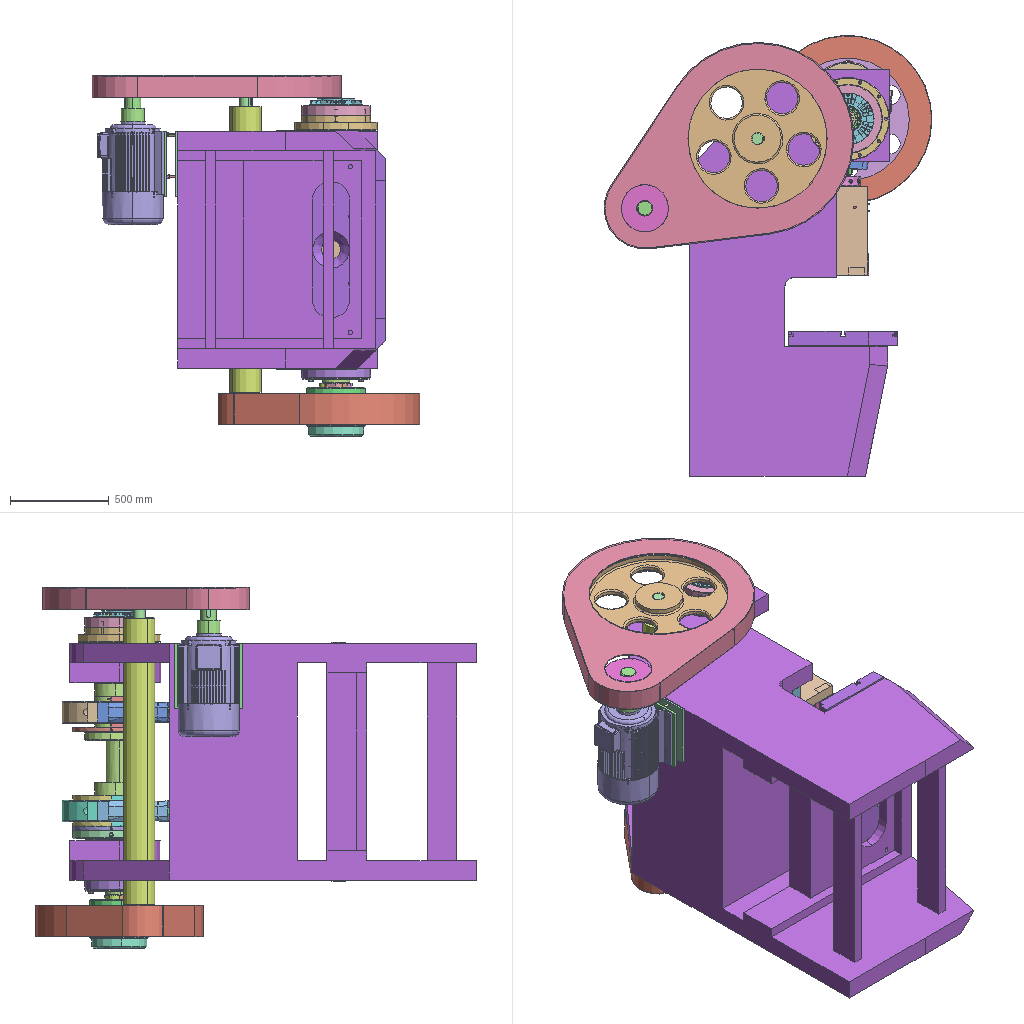Assembly | SolidWorks | 108 different items | 124 placed | box 1659 x 2230 x 1826 mm
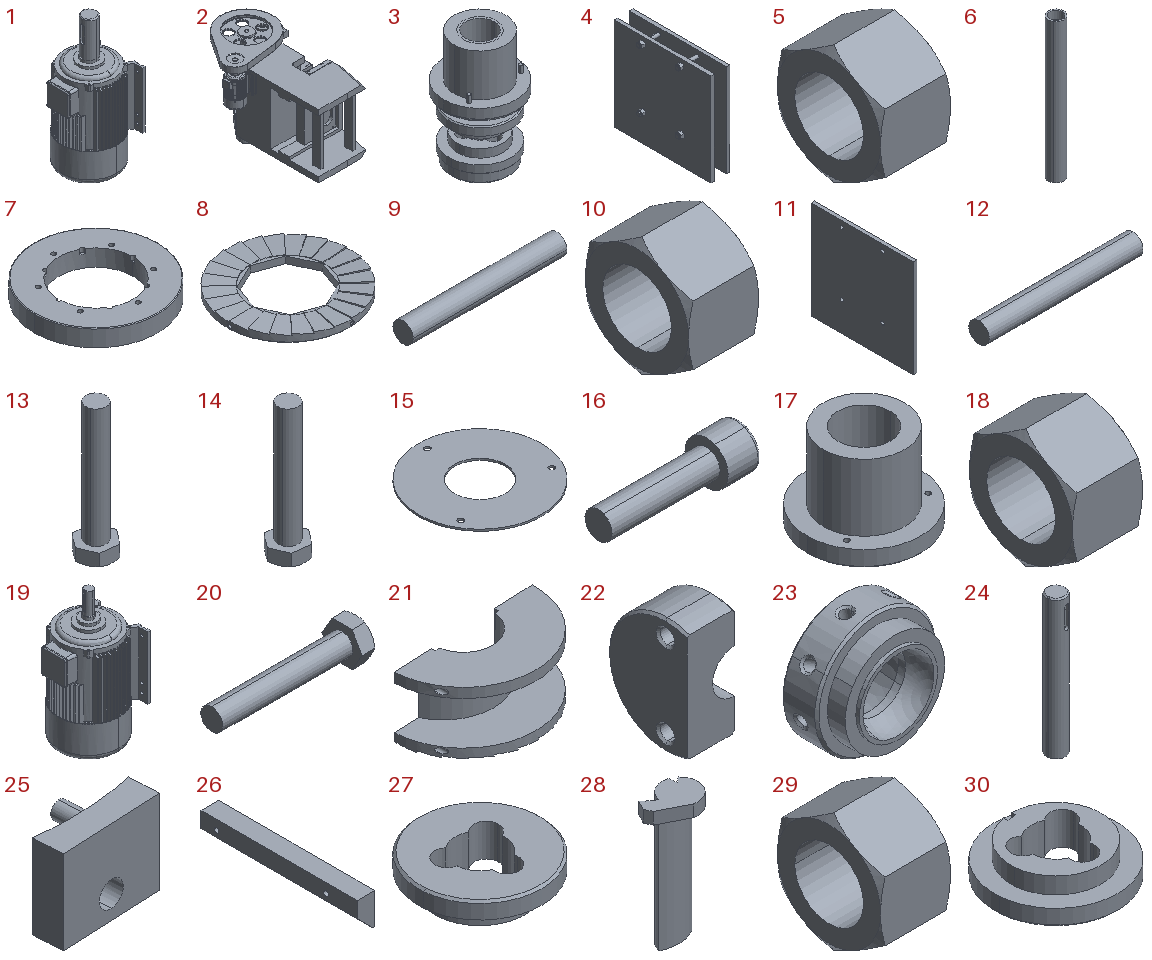Parts list (item | name | quantity | parent item | size | volume | features):
1 | (subassembly) | x1 | in 2 | 340 x 314 x 732 mm | 11771559 mm3 | -
2 | (subassembly) | x1 | - | - | 951819714 mm3 | -
3 | (subassembly) | x1 | in 2 | 350 x 350 x 550 mm | 23094575 mm3 | -
4 | (subassembly) | x1 | in 2 | 90.963 x 344.147 x 330 mm | 2772183 mm3 | -
5 | - | x1 | in 4 | 12.2 x 18 x 20.785 mm | 2031 mm3 | features BaseBody 1
6 | - | x1 | in 2 | 160 x 160 x 1444 mm | 21949365 mm3 | features BaseBody 1
7 | - | x1 | - | 350 x 350 x 48 mm | 2905895 mm3 | features HoleWzd 3, Revolution 1
8 | - | x1 | in 2 | 370 x 370 x 24.255 mm | 1594243 mm3 | features BaseBody 1
9 | - | x1 | in 4 | 90.963 x 12 x 12 mm | 10288 mm3 | features BaseBody 1
10 | - | x1 | in 4 | 12.2 x 18 x 20.785 mm | 2031 mm3 | features BaseBody 1
11 | - | x1 | in 4 | 12 x 344.147 x 330 mm | 1357393 mm3 | features BaseBody 1
12 | - | x1 | in 4 | 90.963 x 12 x 12 mm | 10288 mm3 | features BaseBody 1
13 | - | x1 | in 3 | 27.477 x 25.599 x 100 mm | 20878 mm3 | features BaseBody 1
14 | - | x1 | in 3 | 27.477 x 25.599 x 100 mm | 20878 mm3 | features BaseBody 1
15 | - | x1 | in 3 | 340 x 340 x 5 mm | 374340 mm3 | features BaseBody 1
16 | - | x1 | in 2 | 26 x 8 x 8 mm | 606.379 mm3 | features BaseBody 1
17 | - | x1 | in 3 | 350 x 350 x 255 mm | 9479362 mm3 | features BaseBody 1
18 | - | x1 | in 4 | 12.2 x 18 x 20.785 mm | 2031 mm3 | features BaseBody 1
19 | - | x1 | in 1 | 340 x 314 x 660 mm | 8782416 mm3 | features BaseBody 1
20 | - | x1 | in 2 | 100 x 27.713 x 24 mm | 20878 mm3 | features BaseBody 1
21 | - | x1 | in 2 | 369.799 x 193.623 x 159.255 mm | 2559230 mm3 | features BaseBody 1
22 | - | x1 | in 2 | 65 x 110 x 160 mm | 821212 mm3 | features BaseBody 1
23 | - | x1 | in 2 | 170 x 80 x 170 mm | 1005537 mm3 | features BaseBody 1
24 | - | x1 | in 1 | 80 x 80 x 600 mm | 2989143 mm3 | features BaseBody 1
25 | - | x1 | in 2 | 60.748 x 31.599 x 50 mm | 45964 mm3 | features BaseBody 1
26 | - | x1 | in 2 | 60 x 500 x 100 mm | 2348382 mm3 | features BaseBody 1
27 | - | x1 | in 3 | 300 x 300 x 80 mm | 3048135 mm3 | features BaseBody 1
28 | - | x1 | in 3 | 86.498 x 60 x 220 mm | 320268 mm3 | features BaseBody 1
29 | - | x1 | in 4 | 12.2 x 18 x 20.785 mm | 2031 mm3 | features BaseBody 1
30 | - | x1 | in 3 | 300 x 300 x 80 mm | 3048135 mm3 | features BaseBody 1
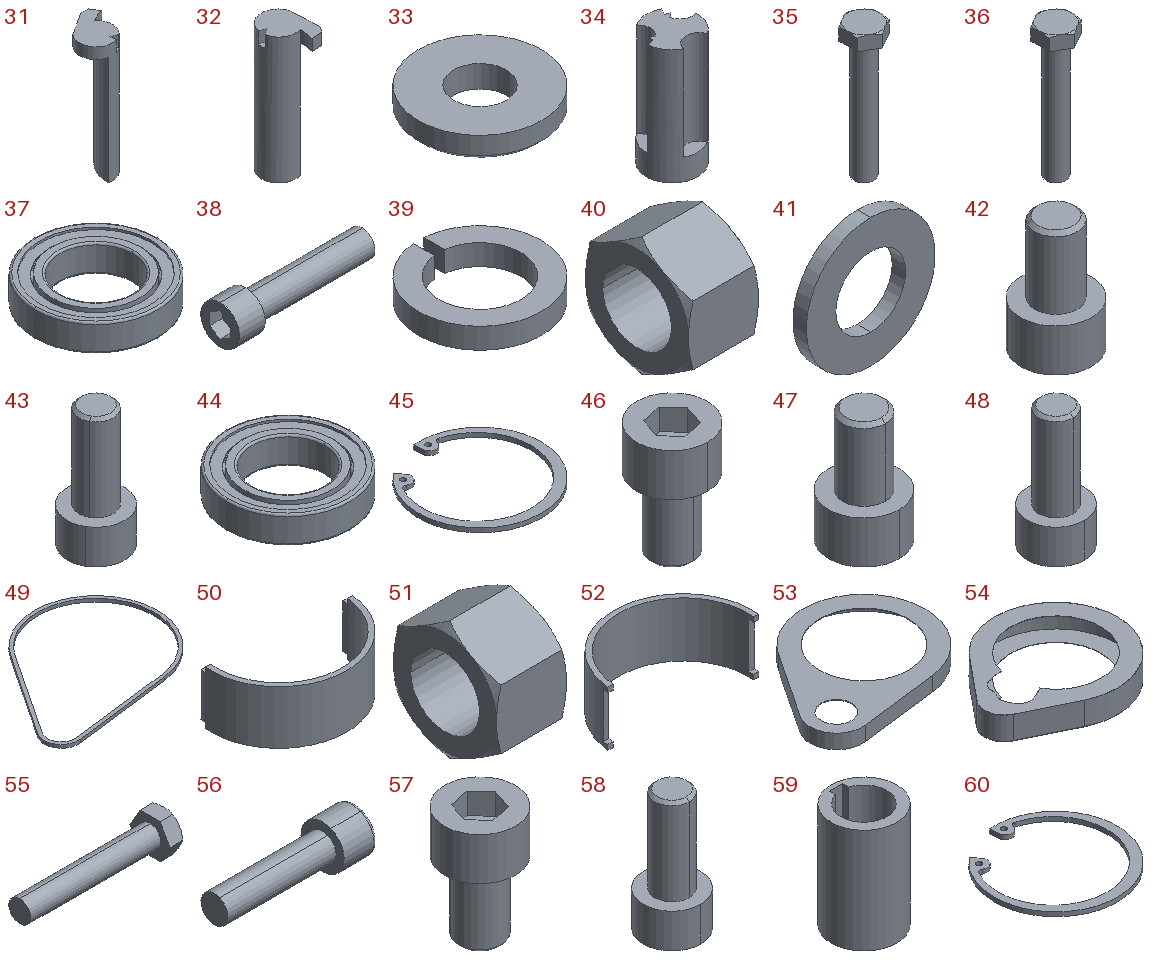31 | - | x1 | in 3 | 72.203 x 77.473 x 220 mm | 320268 mm3 | features BaseBody 1
32 | - | x1 | in 3 | 61.158 x 82.258 x 220 mm | 320268 mm3 | features BaseBody 1
33 | - | x1 | in 3 | 280 x 280 x 50 mm | 2470339 mm3 | features BaseBody 1
34 | - | x1 | in 3 | 120 x 120 x 270 mm | 2222971 mm3 | features BaseBody 1
35 | - | x1 | in 2 | 24 x 27.713 x 100 mm | 20878 mm3 | features BaseBody 1
36 | - | x1 | in 2 | 24 x 27.713 x 100 mm | 20878 mm3 | features BaseBody 1
37 | - | x1 | in 2 | 136 x 136 x 30 mm | 181462 mm3 | features BaseBody 1
38 | - | x2 | in 2 | 67 x 18 x 18 mm | 8742 mm3 | features BaseBody 1
39 | - | x2 | in 2 | 18.367 x 18.334 x 3.1 mm | 444.091 mm3 | features BaseBody 1
40 | - | x1 | in 4 | 12.2 x 18 x 20.785 mm | 2031 mm3 | features BaseBody 1
41 | - | x2 | in 2 | 24 x 2.5 x 24 mm | 799.143 mm3 | features BaseBody 1
42 | - | x7 | in 2 | 20 x 20 x 32 mm | 5504 mm3 | features BaseBody 1
43 | - | x2 | in 2 | 20 x 20 x 42 mm | 6635 mm3 | features BaseBody 1
44 | - | x1 | in 2 | 136 x 136 x 30 mm | 182204 mm3 | features BaseBody 1
45 | - | x1 | in 2 | 145 x 145 x 5 mm | 18463 mm3 | features BaseBody 1
46 | - | x1 | in 2 | 20 x 20 x 32 mm | 5504 mm3 | features BaseBody 1
47 | - | x1 | in 2 | 20 x 20 x 32 mm | 5504 mm3 | features BaseBody 1
48 | - | x1 | in 2 | 20 x 20 x 42 mm | 6635 mm3 | features BaseBody 1
49 | - | x1 | in 2 | 1063 x 845.491 x 20 mm | 1178269 mm3 | features BaseBody 1
50 | - | x1 | in 2 | 279.978 x 162.405 x 110 mm | 484543 mm3 | features BaseBody 1
51 | - | x1 | in 4 | 12.2 x 18 x 20.785 mm | 2031 mm3 | features BaseBody 1
52 | - | x1 | in 2 | 279.443 x 152.477 x 110 mm | 448510 mm3 | features BaseBody 1
53 | - | x1 | in 2 | 1263 x 1045 x 113 mm | 4506392 mm3 | features BaseBody 1
54 | - | x1 | in 2 | 1017 x 850 x 160 mm | 2046242 mm3 | features BaseBody 1
55 | - | x1 | in 2 | 100 x 27.713 x 24 mm | 20878 mm3 | features BaseBody 1
56 | - | x1 | in 2 | 26 x 8 x 8 mm | 606.379 mm3 | features BaseBody 1
57 | - | x1 | in 2 | 20 x 20 x 32 mm | 5504 mm3 | features BaseBody 1
58 | - | x1 | in 2 | 20 x 20 x 42 mm | 6635 mm3 | features BaseBody 1
59 | - | x1 | in 2 | 80 x 80 x 128 mm | 313826 mm3 | features BaseBody 1
60 | - | x1 | in 2 | 145 x 145 x 5 mm | 18463 mm3 | features BaseBody 1
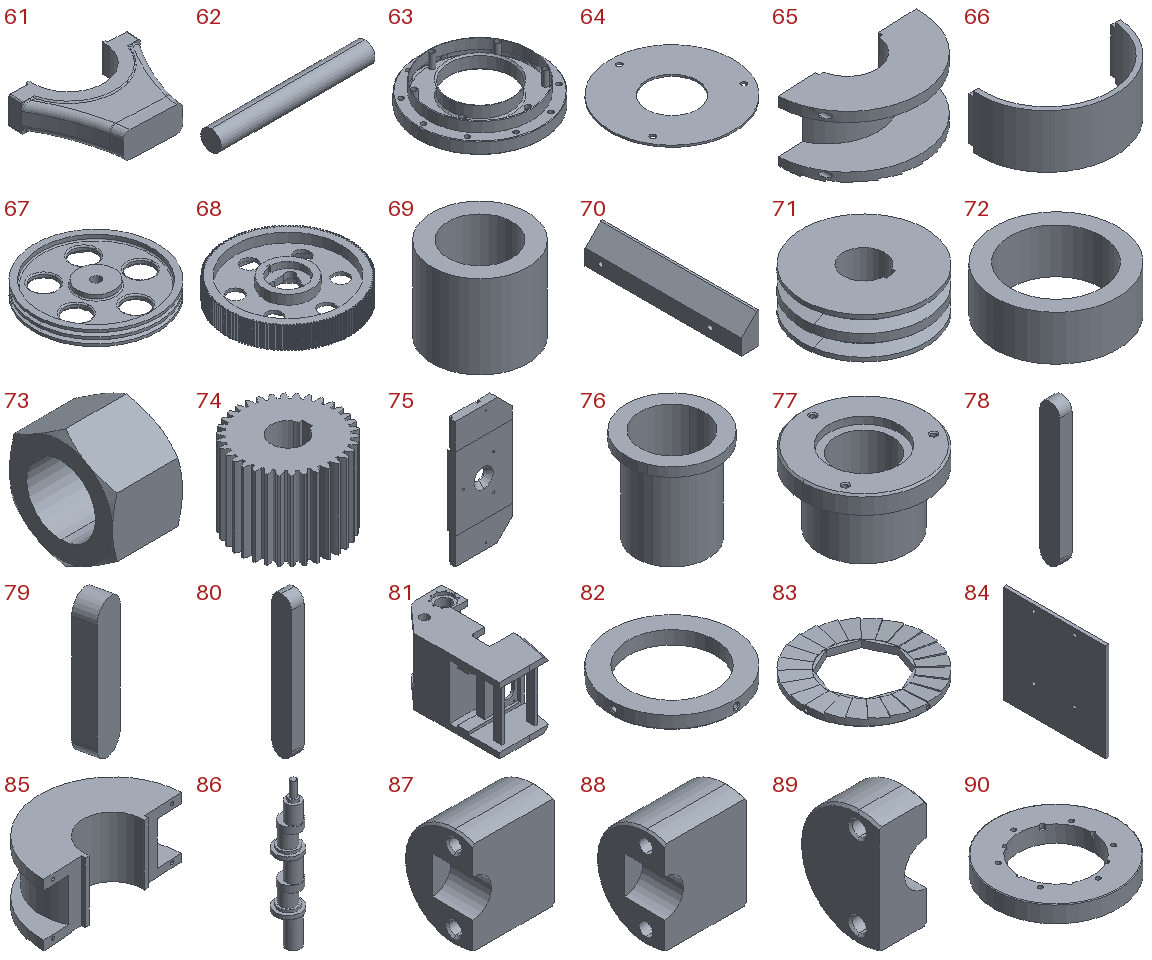61 | - | x1 | in 2 | 455.294 x 369.863 x 110 mm | 8796602 mm3 | features BaseBody 1
62 | - | x1 | in 4 | 90.963 x 12 x 12 mm | 10288 mm3 | features BaseBody 1
63 | - | x1 | in 2 | 420 x 420 x 76 mm | 4501710 mm3 | features BaseBody 1
64 | - | x1 | in 2 | 340 x 340 x 5 mm | 374340 mm3 | features BaseBody 1
65 | - | x1 | in 2 | 369.799 x 193.623 x 159.255 mm | 2559230 mm3 | features BaseBody 1
66 | - | x1 | in 2 | 279.978 x 162.405 x 110 mm | 484543 mm3 | features BaseBody 1
67 | - | x1 | in 2 | 800 x 800 x 96 mm | 19493406 mm3 | features BaseBody 1
68 | - | x1 | in 2 | 789.18 x 789.212 x 140 mm | 25623367 mm3 | features BaseBody 1
69 | - | x1 | in 2 | 120 x 120 x 105 mm | 659734 mm3 | features BaseBody 1
70 | - | x1 | in 2 | 60 x 500 x 100 mm | 2348382 mm3 | features BaseBody 1
71 | - | x1 | in 2 | 240 x 240 x 80 mm | 2615235 mm3 | features BaseBody 1
72 | - | x2 | in 2 | 184 x 184 x 67.2 mm | 810682 mm3 | features BaseBody 1
73 | - | x1 | in 4 | 12.2 x 18 x 20.785 mm | 2031 mm3 | features BaseBody 1
74 | - | x1 | in 2 | 179.662 x 179.997 x 140 mm | 2738233 mm3 | features BaseBody 1
75 | - | x1 | in 2 | 550 x 70 x 1210 mm | 41984418 mm3 | features BaseBody 1
76 | - | x1 | in 2 | 200 x 200 x 205 mm | 1192234 mm3 | features BaseBody 1
77 | - | x1 | in 2 | 350 x 350 x 205 mm | 8030304 mm3 | features BaseBody 1
78 | - | x1 | in 2 | 11.4 x 18 x 130 mm | 25883 mm3 | features BaseBody 1
79 | - | x1 | in 2 | 24.773 x 19.79 x 100 mm | 32490 mm3 | features BaseBody 1
80 | - | x1 | in 2 | 11.4 x 18 x 130 mm | 25883 mm3 | features BaseBody 1
81 | - | x1 | in 2 | 1010 x 2056 x 1200 mm | 587927835 mm3 | features BaseBody 1
82 | - | x1 | in 2 | 370 x 370 x 40 mm | 2151214 mm3 | features BaseBody 1
83 | - | x1 | in 2 | 370 x 370 x 24.255 mm | 1594234 mm3 | features BaseBody 1
84 | - | x1 | in 4 | 12 x 344.147 x 330 mm | 1357393 mm3 | features BaseBody 1
85 | - | x1 | in 2 | 369.799 x 198.951 x 159.255 mm | 5445912 mm3 | features BaseBody 1
86 | - | x1 | in 2 | 250 x 250 x 1419 mm | 25817361 mm3 | features BaseBody 1
87 | - | x1 | in 2 | 130 x 110 x 160 mm | 1738348 mm3 | features BaseBody 1
88 | - | x1 | in 2 | 130 x 110 x 160 mm | 1731219 mm3 | features BaseBody 1
89 | - | x1 | in 2 | 65 x 110 x 160 mm | 821212 mm3 | features BaseBody 1
90 | - | x1 | in 2 | 350 x 350 x 48 mm | 2905895 mm3 | features BaseBody 1
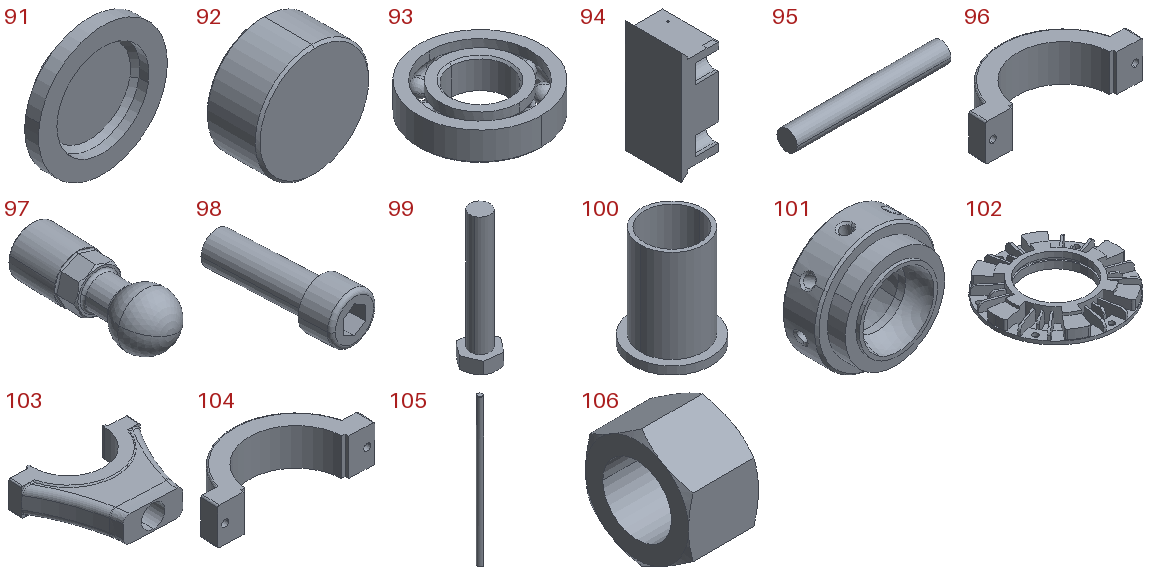91 | - | x1 | in 2 | 140 x 30 x 140 mm | 231551 mm3 | features BaseBody 1
92 | - | x2 | in 2 | 140 x 65 x 140 mm | 687379 mm3 | features BaseBody 1
93 | - | x4 | in 2 | 130 x 130 x 31 mm | 224912 mm3 | features BaseBody 1
94 | - | x1 | in 2 | 300 x 450 x 900 mm | 94683231 mm3 | features BaseBody 1
95 | - | x1 | in 4 | 90.963 x 12 x 12 mm | 10288 mm3 | features BaseBody 1
96 | - | x1 | in 2 | 454.449 x 198.703 x 110 mm | 3221578 mm3 | features BaseBody 1
97 | - | x2 | in 2 | 103.341 x 271.49 x 100 mm | 1435475 mm3 | features BaseBody 1
98 | - | x1 | in 2 | 12.314 x 33.385 x 12 mm | 1904 mm3 | features BaseBody 1
99 | - | x1 | in 3 | 27.477 x 25.599 x 100 mm | 20878 mm3 | features BaseBody 1
100 | - | x1 | in 3 | 200 x 200 x 255 mm | 1427854 mm3 | features BaseBody 1
101 | - | x1 | in 2 | 170 x 80 x 170 mm | 1005537 mm3 | features BaseBody 1
102 | - | x1 | in 2 | 264 x 264 x 33 mm | 629435 mm3 | features BaseBody 1
103 | - | x1 | in 2 | 455.294 x 369.863 x 110 mm | 7905953 mm3 | features BaseBody 1
104 | - | x1 | in 2 | 454.449 x 198.703 x 110 mm | 3221578 mm3 | features BaseBody 1
105 | - | x1 | in 2 | 60 x 60 x 1739 mm | 4902443 mm3 | features BaseBody 1
106 | - | x1 | in 4 | 12.2 x 18 x 20.785 mm | 2031 mm3 | features BaseBody 1
107 | Belt | x1 | - | - | - | -
108 | Cover Plate | x1 | - | - | - | -